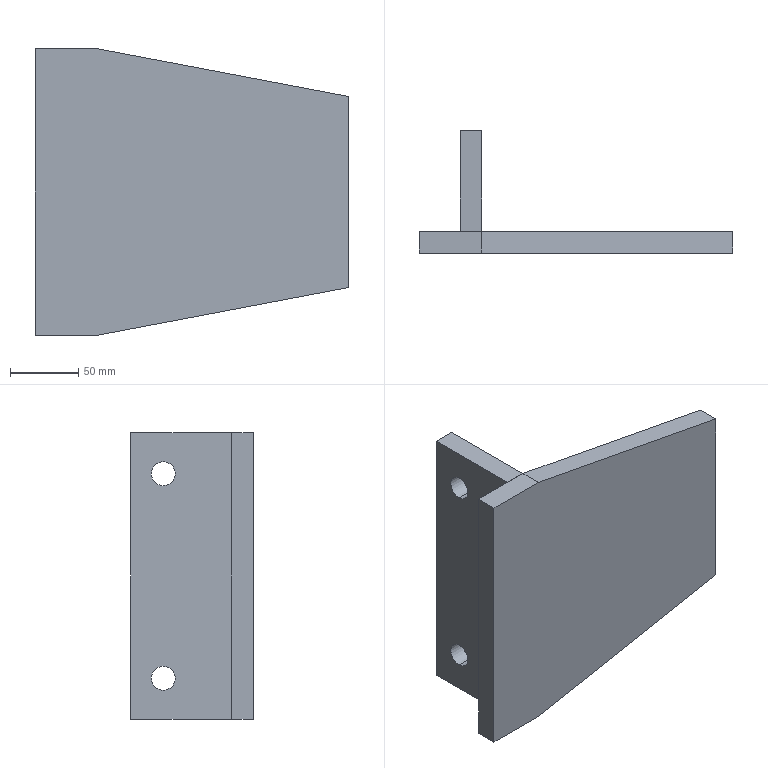Part | SolidWorks | features MirrorStock 1 | 2 solids | 18 faces | box 230 x 90 x 210 mm | volume 910703 mm3 | plane 14 | cylinder 4 | commonest cylinder face diameters 17.5 x4
STEP:
#1=CARTESIAN_POINT('',(46.,0.,105.));
#2=VERTEX_POINT('',#1);
#3=CARTESIAN_POINT('',(0.,0.,105.));
#4=VERTEX_POINT('',#3);
#5=CARTESIAN_POINT('',(46.,0.,105.));
#6=DIRECTION('',(-1.,0.,0.));
#7=VECTOR('',#6,1000.);
#8=LINE('',#5,#7);
#9=EDGE_CURVE('',#2,#4,#8,.T.);
#10=ORIENTED_EDGE('',*,*,#9,.F.);
#11=CARTESIAN_POINT('',(46.,16.,105.));
#12=VERTEX_POINT('',#11);
#13=CARTESIAN_POINT('',(46.,16.,105.));
#14=DIRECTION('',(0.,-1.,0.));
#15=VECTOR('',#14,1000.);
#16=LINE('',#13,#15);
#17=EDGE_CURVE('',#12,#2,#16,.T.);
#18=ORIENTED_EDGE('',*,*,#17,.F.);
#19=CARTESIAN_POINT('',(0.,16.,105.));
#20=VERTEX_POINT('',#19);
#21=CARTESIAN_POINT('',(46.,16.,105.));
#22=DIRECTION('',(-1.,0.,0.));
#23=VECTOR('',#22,1000.);
#24=LINE('',#21,#23);
#25=EDGE_CURVE('',#12,#20,#24,.T.);
#26=ORIENTED_EDGE('',*,*,#25,.T.);
#27=CARTESIAN_POINT('',(0.,16.,105.));
#28=DIRECTION('',(0.,-1.,0.));
#29=VECTOR('',#28,1000.);
#30=LINE('',#27,#29);
#31=EDGE_CURVE('',#20,#4,#30,.T.);
#32=ORIENTED_EDGE('',*,*,#31,.T.);
#33=EDGE_LOOP('',(#10,#18,#26,#32));
#34=FACE_OUTER_BOUND('',#33,.T.);
#35=CARTESIAN_POINT('',(46.,16.,105.));
#36=DIRECTION('',(0.,0.,-1.));
#37=DIRECTION('',(1.,0.,0.));
#38=AXIS2_PLACEMENT_3D('',#35,#36,#37);
#39=PLANE('',#38);
#40=ADVANCED_FACE('',(#34),#39,.F.);
#41=CARTESIAN_POINT('',(0.,0.,-105.));
#42=VERTEX_POINT('',#41);
#43=CARTESIAN_POINT('',(0.,0.,105.));
#44=DIRECTION('',(0.,0.,-1.));
#45=VECTOR('',#44,1000.);
#46=LINE('',#43,#45);
#47=EDGE_CURVE('',#4,#42,#46,.T.);
#48=ORIENTED_EDGE('',*,*,#47,.F.);
#49=ORIENTED_EDGE('',*,*,#31,.F.);
#50=CARTESIAN_POINT('',(0.,16.,-105.));
#51=VERTEX_POINT('',#50);
#52=CARTESIAN_POINT('',(0.,16.,105.));
#53=DIRECTION('',(0.,0.,-1.));
#54=VECTOR('',#53,1000.);
#55=LINE('',#52,#54);
#56=EDGE_CURVE('',#20,#51,#55,.T.);
#57=ORIENTED_EDGE('',*,*,#56,.T.);
#58=CARTESIAN_POINT('',(0.,16.,-105.));
#59=DIRECTION('',(0.,-1.,0.));
#60=VECTOR('',#59,1000.);
#61=LINE('',#58,#60);
#62=EDGE_CURVE('',#51,#42,#61,.T.);
#63=ORIENTED_EDGE('',*,*,#62,.T.);
#64=EDGE_LOOP('',(#48,#49,#57,#63));
#65=FACE_OUTER_BOUND('',#64,.T.);
#66=CARTESIAN_POINT('',(0.,16.,105.));
#67=DIRECTION('',(1.,0.,0.));
#68=DIRECTION('',(0.,0.,1.));
#69=AXIS2_PLACEMENT_3D('',#66,#67,#68);
#70=PLANE('',#69);
#71=ADVANCED_FACE('',(#65),#70,.F.);
#72=CARTESIAN_POINT('',(46.,0.,-105.));
#73=VERTEX_POINT('',#72);
#74=CARTESIAN_POINT('',(46.,0.,-105.));
#75=DIRECTION('',(1.,0.,0.));
#76=VECTOR('',#75,1000.);
#77=LINE('',#74,#76);
#78=EDGE_CURVE('',#42,#73,#77,.T.);
#79=ORIENTED_EDGE('',*,*,#78,.F.);
#80=ORIENTED_EDGE('',*,*,#62,.F.);
#81=CARTESIAN_POINT('',(46.,16.,-105.));
#82=VERTEX_POINT('',#81);
#83=CARTESIAN_POINT('',(46.,16.,-105.));
#84=DIRECTION('',(1.,0.,0.));
#85=VECTOR('',#84,1000.);
#86=LINE('',#83,#85);
#87=EDGE_CURVE('',#51,#82,#86,.T.);
#88=ORIENTED_EDGE('',*,*,#87,.T.);
#89=CARTESIAN_POINT('',(46.,16.,-105.));
#90=DIRECTION('',(0.,-1.,0.));
#91=VECTOR('',#90,1000.);
#92=LINE('',#89,#91);
#93=EDGE_CURVE('',#82,#73,#92,.T.);
#94=ORIENTED_EDGE('',*,*,#93,.T.);
#95=EDGE_LOOP('',(#79,#80,#88,#94));
#96=FACE_OUTER_BOUND('',#95,.T.);
#97=CARTESIAN_POINT('',(46.,16.,-105.));
#98=DIRECTION('',(0.,0.,1.));
#99=DIRECTION('',(-1.,0.,0.));
#100=AXIS2_PLACEMENT_3D('',#97,#98,#99);
#101=PLANE('',#100);
#102=ADVANCED_FACE('',(#96),#101,.F.);
#103=CARTESIAN_POINT('',(230.,0.,-70.));
#104=VERTEX_POINT('',#103);
#105=CARTESIAN_POINT('',(230.,0.,-70.));
#106=DIRECTION('',(0.9824,0.,0.1869));
#107=VECTOR('',#106,1000.);
#108=LINE('',#105,#107);
#109=EDGE_CURVE('',#73,#104,#108,.T.);
#110=ORIENTED_EDGE('',*,*,#109,.F.);
#111=ORIENTED_EDGE('',*,*,#93,.F.);
#112=CARTESIAN_POINT('',(230.,16.,-70.));
#113=VERTEX_POINT('',#112);
#114=CARTESIAN_POINT('',(230.,16.,-70.));
#115=DIRECTION('',(0.9824,0.,0.1869));
#116=VECTOR('',#115,1000.);
#117=LINE('',#114,#116);
#118=EDGE_CURVE('',#82,#113,#117,.T.);
#119=ORIENTED_EDGE('',*,*,#118,.T.);
#120=CARTESIAN_POINT('',(230.,16.,-70.));
#121=DIRECTION('',(0.,-1.,0.));
#122=VECTOR('',#121,1000.);
#123=LINE('',#120,#122);
#124=EDGE_CURVE('',#113,#104,#123,.T.);
#125=ORIENTED_EDGE('',*,*,#124,.T.);
#126=EDGE_LOOP('',(#110,#111,#119,#125));
#127=FACE_OUTER_BOUND('',#126,.T.);
#128=CARTESIAN_POINT('',(230.,16.,-70.));
#129=DIRECTION('',(-0.1869,0.,0.9824));
#130=DIRECTION('',(-0.9824,0.,-0.1869));
#131=AXIS2_PLACEMENT_3D('',#128,#129,#130);
#132=PLANE('',#131);
#133=ADVANCED_FACE('',(#127),#132,.F.);
#134=CARTESIAN_POINT('',(230.,0.,70.));
#135=VERTEX_POINT('',#134);
#136=CARTESIAN_POINT('',(230.,0.,-70.));
#137=DIRECTION('',(0.,0.,1.));
#138=VECTOR('',#137,1000.);
#139=LINE('',#136,#138);
#140=EDGE_CURVE('',#104,#135,#139,.T.);
#141=ORIENTED_EDGE('',*,*,#140,.F.);
#142=ORIENTED_EDGE('',*,*,#124,.F.);
#143=CARTESIAN_POINT('',(230.,16.,70.));
#144=VERTEX_POINT('',#143);
#145=CARTESIAN_POINT('',(230.,16.,-70.));
#146=DIRECTION('',(0.,0.,1.));
#147=VECTOR('',#146,1000.);
#148=LINE('',#145,#147);
#149=EDGE_CURVE('',#113,#144,#148,.T.);
#150=ORIENTED_EDGE('',*,*,#149,.T.);
#151=CARTESIAN_POINT('',(230.,16.,70.));
#152=DIRECTION('',(0.,-1.,0.));
#153=VECTOR('',#152,1000.);
#154=LINE('',#151,#153);
#155=EDGE_CURVE('',#144,#135,#154,.T.);
#156=ORIENTED_EDGE('',*,*,#155,.T.);
#157=EDGE_LOOP('',(#141,#142,#150,#156));
#158=FACE_OUTER_BOUND('',#157,.T.);
#159=CARTESIAN_POINT('',(230.,16.,-70.));
#160=DIRECTION('',(-1.,0.,0.));
#161=DIRECTION('',(0.,0.,-1.));
#162=AXIS2_PLACEMENT_3D('',#159,#160,#161);
#163=PLANE('',#162);
#164=ADVANCED_FACE('',(#158),#163,.F.);
#165=CARTESIAN_POINT('',(230.,0.,70.));
#166=DIRECTION('',(-0.9824,0.,0.1869));
#167=VECTOR('',#166,1000.);
#168=LINE('',#165,#167);
#169=EDGE_CURVE('',#135,#2,#168,.T.);
#170=ORIENTED_EDGE('',*,*,#169,.F.);
#171=ORIENTED_EDGE('',*,*,#155,.F.);
#172=CARTESIAN_POINT('',(230.,16.,70.));
#173=DIRECTION('',(-0.9824,0.,0.1869));
#174=VECTOR('',#173,1000.);
#175=LINE('',#172,#174);
#176=EDGE_CURVE('',#144,#12,#175,.T.);
#177=ORIENTED_EDGE('',*,*,#176,.T.);
#178=ORIENTED_EDGE('',*,*,#17,.T.);
#179=EDGE_LOOP('',(#170,#171,#177,#178));
#180=FACE_OUTER_BOUND('',#179,.T.);
#181=CARTESIAN_POINT('',(230.,16.,70.));
#182=DIRECTION('',(-0.1869,0.,-0.9824));
#183=DIRECTION('',(0.9824,0.,-0.1869));
#184=AXIS2_PLACEMENT_3D('',#181,#182,#183);
#185=PLANE('',#184);
#186=ADVANCED_FACE('',(#180),#185,.F.);
#187=ORIENTED_EDGE('',*,*,#25,.F.);
#188=ORIENTED_EDGE('',*,*,#176,.F.);
#189=ORIENTED_EDGE('',*,*,#149,.F.);
#190=ORIENTED_EDGE('',*,*,#118,.F.);
#191=ORIENTED_EDGE('',*,*,#87,.F.);
#192=ORIENTED_EDGE('',*,*,#56,.F.);
#193=EDGE_LOOP('',(#187,#188,#189,#190,#191,#192));
#194=FACE_OUTER_BOUND('',#193,.T.);
#195=CARTESIAN_POINT('',(0.,16.,0.));
#196=DIRECTION('',(0.,1.,0.));
#197=DIRECTION('',(0.,0.,-1.));
#198=AXIS2_PLACEMENT_3D('',#195,#196,#197);
#199=PLANE('',#198);
#200=ADVANCED_FACE('',(#194),#199,.T.);
#201=ORIENTED_EDGE('',*,*,#9,.T.);
#202=ORIENTED_EDGE('',*,*,#47,.T.);
#203=ORIENTED_EDGE('',*,*,#78,.T.);
#204=ORIENTED_EDGE('',*,*,#109,.T.);
#205=ORIENTED_EDGE('',*,*,#140,.T.);
#206=ORIENTED_EDGE('',*,*,#169,.T.);
#207=EDGE_LOOP('',(#201,#202,#203,#204,#205,#206));
#208=FACE_OUTER_BOUND('',#207,.T.);
#209=CARTESIAN_POINT('',(0.,0.,0.));
#210=DIRECTION('',(0.,1.,0.));
#211=DIRECTION('',(0.,0.,-1.));
#212=AXIS2_PLACEMENT_3D('',#209,#210,#211);
#213=PLANE('',#212);
#214=ADVANCED_FACE('',(#208),#213,.F.);
#215=CLOSED_SHELL('',(#40,#71,#102,#133,#164,#186,#200,#214));
#216=MANIFOLD_SOLID_BREP('',#215);
#217=CARTESIAN_POINT('',(46.,66.,66.25));
#218=VERTEX_POINT('',#217);
#219=CARTESIAN_POINT('',(46.,66.,83.75));
#220=VERTEX_POINT('',#219);
#221=CARTESIAN_POINT('',(46.,66.,75.));
#222=DIRECTION('',(1.,0.,0.));
#223=DIRECTION('',(0.,0.,-1.));
#224=AXIS2_PLACEMENT_3D('',#221,#222,#223);
#225=CIRCLE('',#224,8.75);
#226=EDGE_CURVE('',#218,#220,#225,.T.);
#227=ORIENTED_EDGE('',*,*,#226,.T.);
#228=CARTESIAN_POINT('',(30.,66.,83.75));
#229=VERTEX_POINT('',#228);
#230=CARTESIAN_POINT('',(30.,66.,83.75));
#231=DIRECTION('',(-1.,0.,0.));
#232=VECTOR('',#231,1000.);
#233=LINE('',#230,#232);
#234=EDGE_CURVE('',#220,#229,#233,.T.);
#235=ORIENTED_EDGE('',*,*,#234,.T.);
#236=CARTESIAN_POINT('',(30.,66.,66.25));
#237=VERTEX_POINT('',#236);
#238=CARTESIAN_POINT('',(30.,66.,75.));
#239=DIRECTION('',(1.,0.,0.));
#240=DIRECTION('',(0.,0.,-1.));
#241=AXIS2_PLACEMENT_3D('',#238,#239,#240);
#242=CIRCLE('',#241,8.75);
#243=EDGE_CURVE('',#237,#229,#242,.T.);
#244=ORIENTED_EDGE('',*,*,#243,.F.);
#245=CARTESIAN_POINT('',(30.,66.,66.25));
#246=DIRECTION('',(-1.,0.,0.));
#247=VECTOR('',#246,1000.);
#248=LINE('',#245,#247);
#249=EDGE_CURVE('',#218,#237,#248,.T.);
#250=ORIENTED_EDGE('',*,*,#249,.F.);
#251=EDGE_LOOP('',(#227,#235,#244,#250));
#252=FACE_OUTER_BOUND('',#251,.T.);
#253=CARTESIAN_POINT('',(30.,66.,75.));
#254=DIRECTION('',(-1.,0.,0.));
#255=DIRECTION('',(0.,0.,-1.));
#256=AXIS2_PLACEMENT_3D('',#253,#254,#255);
#257=CYLINDRICAL_SURFACE('',#256,8.75);
#258=ADVANCED_FACE('',(#252),#257,.F.);
#259=CARTESIAN_POINT('',(46.,66.,-83.75));
#260=VERTEX_POINT('',#259);
#261=CARTESIAN_POINT('',(46.,66.,-66.25));
#262=VERTEX_POINT('',#261);
#263=CARTESIAN_POINT('',(46.,66.,-75.));
#264=DIRECTION('',(1.,0.,0.));
#265=DIRECTION('',(0.,0.,-1.));
#266=AXIS2_PLACEMENT_3D('',#263,#264,#265);
#267=CIRCLE('',#266,8.75);
#268=EDGE_CURVE('',#260,#262,#267,.T.);
#269=ORIENTED_EDGE('',*,*,#268,.T.);
#270=CARTESIAN_POINT('',(30.,66.,-66.25));
#271=VERTEX_POINT('',#270);
#272=CARTESIAN_POINT('',(30.,66.,-66.25));
#273=DIRECTION('',(-1.,0.,0.));
#274=VECTOR('',#273,1000.);
#275=LINE('',#272,#274);
#276=EDGE_CURVE('',#262,#271,#275,.T.);
#277=ORIENTED_EDGE('',*,*,#276,.T.);
#278=CARTESIAN_POINT('',(30.,66.,-83.75));
#279=VERTEX_POINT('',#278);
#280=CARTESIAN_POINT('',(30.,66.,-75.));
#281=DIRECTION('',(1.,0.,0.));
#282=DIRECTION('',(0.,0.,-1.));
#283=AXIS2_PLACEMENT_3D('',#280,#281,#282);
#284=CIRCLE('',#283,8.75);
#285=EDGE_CURVE('',#279,#271,#284,.T.);
#286=ORIENTED_EDGE('',*,*,#285,.F.);
#287=CARTESIAN_POINT('',(30.,66.,-83.75));
#288=DIRECTION('',(-1.,0.,0.));
#289=VECTOR('',#288,1000.);
#290=LINE('',#287,#289);
#291=EDGE_CURVE('',#260,#279,#290,.T.);
#292=ORIENTED_EDGE('',*,*,#291,.F.);
#293=EDGE_LOOP('',(#269,#277,#286,#292));
#294=FACE_OUTER_BOUND('',#293,.T.);
#295=CARTESIAN_POINT('',(30.,66.,-75.));
#296=DIRECTION('',(-1.,0.,0.));
#297=DIRECTION('',(0.,0.,-1.));
#298=AXIS2_PLACEMENT_3D('',#295,#296,#297);
#299=CYLINDRICAL_SURFACE('',#298,8.75);
#300=ADVANCED_FACE('',(#294),#299,.F.);
#301=ORIENTED_EDGE('',*,*,#226,.F.);
#302=CARTESIAN_POINT('',(46.,66.,75.));
#303=DIRECTION('',(1.,0.,0.));
#304=DIRECTION('',(0.,0.,-1.));
#305=AXIS2_PLACEMENT_3D('',#302,#303,#304);
#306=CIRCLE('',#305,8.75);
#307=EDGE_CURVE('',#220,#218,#306,.T.);
#308=ORIENTED_EDGE('',*,*,#307,.F.);
#309=EDGE_LOOP('',(#301,#308));
#310=FACE_BOUND('',#309,.T.);
#311=ORIENTED_EDGE('',*,*,#268,.F.);
#312=CARTESIAN_POINT('',(46.,66.,-75.));
#313=DIRECTION('',(1.,0.,0.));
#314=DIRECTION('',(0.,0.,-1.));
#315=AXIS2_PLACEMENT_3D('',#312,#313,#314);
#316=CIRCLE('',#315,8.75);
#317=EDGE_CURVE('',#262,#260,#316,.T.);
#318=ORIENTED_EDGE('',*,*,#317,.F.);
#319=EDGE_LOOP('',(#311,#318));
#320=FACE_BOUND('',#319,.T.);
#321=CARTESIAN_POINT('',(46.,16.,-105.));
#322=VERTEX_POINT('',#321);
#323=CARTESIAN_POINT('',(46.,16.,105.));
#324=VERTEX_POINT('',#323);
#325=CARTESIAN_POINT('',(46.,16.,105.));
#326=DIRECTION('',(0.,0.,1.));
#327=VECTOR('',#326,1000.);
#328=LINE('',#325,#327);
#329=EDGE_CURVE('',#322,#324,#328,.T.);
#330=ORIENTED_EDGE('',*,*,#329,.F.);
#331=CARTESIAN_POINT('',(46.,90.,-105.));
#332=VERTEX_POINT('',#331);
#333=CARTESIAN_POINT('',(46.,90.,-105.));
#334=DIRECTION('',(0.,-1.,0.));
#335=VECTOR('',#334,1000.);
#336=LINE('',#333,#335);
#337=EDGE_CURVE('',#332,#322,#336,.T.);
#338=ORIENTED_EDGE('',*,*,#337,.F.);
#339=CARTESIAN_POINT('',(46.,90.,105.));
#340=VERTEX_POINT('',#339);
#341=CARTESIAN_POINT('',(46.,90.,105.));
#342=DIRECTION('',(0.,0.,1.));
#343=VECTOR('',#342,1000.);
#344=LINE('',#341,#343);
#345=EDGE_CURVE('',#332,#340,#344,.T.);
#346=ORIENTED_EDGE('',*,*,#345,.T.);
#347=CARTESIAN_POINT('',(46.,90.,105.));
#348=DIRECTION('',(0.,-1.,0.));
#349=VECTOR('',#348,1000.);
#350=LINE('',#347,#349);
#351=EDGE_CURVE('',#340,#324,#350,.T.);
#352=ORIENTED_EDGE('',*,*,#351,.T.);
#353=EDGE_LOOP('',(#330,#338,#346,#352));
#354=FACE_OUTER_BOUND('',#353,.T.);
#355=CARTESIAN_POINT('',(46.,90.,105.));
#356=DIRECTION('',(-1.,0.,0.));
#357=DIRECTION('',(0.,0.,-1.));
#358=AXIS2_PLACEMENT_3D('',#355,#356,#357);
#359=PLANE('',#358);
#360=ADVANCED_FACE('',(#310,#320,#354),#359,.F.);
#361=CARTESIAN_POINT('',(30.,16.,105.));
#362=VERTEX_POINT('',#361);
#363=CARTESIAN_POINT('',(46.,16.,105.));
#364=DIRECTION('',(-1.,0.,0.));
#365=VECTOR('',#364,1000.);
#366=LINE('',#363,#365);
#367=EDGE_CURVE('',#324,#362,#366,.T.);
#368=ORIENTED_EDGE('',*,*,#367,.F.);
#369=ORIENTED_EDGE('',*,*,#351,.F.);
#370=CARTESIAN_POINT('',(30.,90.,105.));
#371=VERTEX_POINT('',#370);
#372=CARTESIAN_POINT('',(46.,90.,105.));
#373=DIRECTION('',(-1.,0.,0.));
#374=VECTOR('',#373,1000.);
#375=LINE('',#372,#374);
#376=EDGE_CURVE('',#340,#371,#375,.T.);
#377=ORIENTED_EDGE('',*,*,#376,.T.);
#378=CARTESIAN_POINT('',(30.,90.,105.));
#379=DIRECTION('',(0.,-1.,0.));
#380=VECTOR('',#379,1000.);
#381=LINE('',#378,#380);
#382=EDGE_CURVE('',#371,#362,#381,.T.);
#383=ORIENTED_EDGE('',*,*,#382,.T.);
#384=EDGE_LOOP('',(#368,#369,#377,#383));
#385=FACE_OUTER_BOUND('',#384,.T.);
#386=CARTESIAN_POINT('',(46.,90.,105.));
#387=DIRECTION('',(0.,0.,-1.));
#388=DIRECTION('',(1.,0.,0.));
#389=AXIS2_PLACEMENT_3D('',#386,#387,#388);
#390=PLANE('',#389);
#391=ADVANCED_FACE('',(#385),#390,.F.);
#392=ORIENTED_EDGE('',*,*,#243,.T.);
#393=CARTESIAN_POINT('',(30.,66.,75.));
#394=DIRECTION('',(1.,0.,0.));
#395=DIRECTION('',(0.,0.,-1.));
#396=AXIS2_PLACEMENT_3D('',#393,#394,#395);
#397=CIRCLE('',#396,8.75);
#398=EDGE_CURVE('',#229,#237,#397,.T.);
#399=ORIENTED_EDGE('',*,*,#398,.T.);
#400=EDGE_LOOP('',(#392,#399));
#401=FACE_BOUND('',#400,.T.);
#402=ORIENTED_EDGE('',*,*,#285,.T.);
#403=CARTESIAN_POINT('',(30.,66.,-75.));
#404=DIRECTION('',(1.,0.,0.));
#405=DIRECTION('',(0.,0.,-1.));
#406=AXIS2_PLACEMENT_3D('',#403,#404,#405);
#407=CIRCLE('',#406,8.75);
#408=EDGE_CURVE('',#271,#279,#407,.T.);
#409=ORIENTED_EDGE('',*,*,#408,.T.);
#410=EDGE_LOOP('',(#402,#409));
#411=FACE_BOUND('',#410,.T.);
#412=CARTESIAN_POINT('',(30.,16.,-105.));
#413=VERTEX_POINT('',#412);
#414=CARTESIAN_POINT('',(30.,16.,105.));
#415=DIRECTION('',(0.,0.,-1.));
#416=VECTOR('',#415,1000.);
#417=LINE('',#414,#416);
#418=EDGE_CURVE('',#362,#413,#417,.T.);
#419=ORIENTED_EDGE('',*,*,#418,.F.);
#420=ORIENTED_EDGE('',*,*,#382,.F.);
#421=CARTESIAN_POINT('',(30.,90.,-105.));
#422=VERTEX_POINT('',#421);
#423=CARTESIAN_POINT('',(30.,90.,105.));
#424=DIRECTION('',(0.,0.,-1.));
#425=VECTOR('',#424,1000.);
#426=LINE('',#423,#425);
#427=EDGE_CURVE('',#371,#422,#426,.T.);
#428=ORIENTED_EDGE('',*,*,#427,.T.);
#429=CARTESIAN_POINT('',(30.,90.,-105.));
#430=DIRECTION('',(0.,-1.,0.));
#431=VECTOR('',#430,1000.);
#432=LINE('',#429,#431);
#433=EDGE_CURVE('',#422,#413,#432,.T.);
#434=ORIENTED_EDGE('',*,*,#433,.T.);
#435=EDGE_LOOP('',(#419,#420,#428,#434));
#436=FACE_OUTER_BOUND('',#435,.T.);
#437=CARTESIAN_POINT('',(30.,90.,105.));
#438=DIRECTION('',(1.,0.,0.));
#439=DIRECTION('',(0.,0.,1.));
#440=AXIS2_PLACEMENT_3D('',#437,#438,#439);
#441=PLANE('',#440);
#442=ADVANCED_FACE('',(#401,#411,#436),#441,.F.);
#443=CARTESIAN_POINT('',(46.,16.,-105.));
#444=DIRECTION('',(1.,0.,0.));
#445=VECTOR('',#444,1000.);
#446=LINE('',#443,#445);
#447=EDGE_CURVE('',#413,#322,#446,.T.);
#448=ORIENTED_EDGE('',*,*,#447,.F.);
#449=ORIENTED_EDGE('',*,*,#433,.F.);
#450=CARTESIAN_POINT('',(46.,90.,-105.));
#451=DIRECTION('',(1.,0.,0.));
#452=VECTOR('',#451,1000.);
#453=LINE('',#450,#452);
#454=EDGE_CURVE('',#422,#332,#453,.T.);
#455=ORIENTED_EDGE('',*,*,#454,.T.);
#456=ORIENTED_EDGE('',*,*,#337,.T.);
#457=EDGE_LOOP('',(#448,#449,#455,#456));
#458=FACE_OUTER_BOUND('',#457,.T.);
#459=CARTESIAN_POINT('',(46.,90.,-105.));
#460=DIRECTION('',(0.,0.,1.));
#461=DIRECTION('',(-1.,0.,0.));
#462=AXIS2_PLACEMENT_3D('',#459,#460,#461);
#463=PLANE('',#462);
#464=ADVANCED_FACE('',(#458),#463,.F.);
#465=ORIENTED_EDGE('',*,*,#345,.F.);
#466=ORIENTED_EDGE('',*,*,#454,.F.);
#467=ORIENTED_EDGE('',*,*,#427,.F.);
#468=ORIENTED_EDGE('',*,*,#376,.F.);
#469=EDGE_LOOP('',(#465,#466,#467,#468));
#470=FACE_OUTER_BOUND('',#469,.T.);
#471=CARTESIAN_POINT('',(0.,90.,0.));
#472=DIRECTION('',(0.,-1.,0.));
#473=DIRECTION('',(0.,0.,1.));
#474=AXIS2_PLACEMENT_3D('',#471,#472,#473);
#475=PLANE('',#474);
#476=ADVANCED_FACE('',(#470),#475,.F.);
#477=ORIENTED_EDGE('',*,*,#329,.T.);
#478=ORIENTED_EDGE('',*,*,#367,.T.);
#479=ORIENTED_EDGE('',*,*,#418,.T.);
#480=ORIENTED_EDGE('',*,*,#447,.T.);
#481=EDGE_LOOP('',(#477,#478,#479,#480));
#482=FACE_OUTER_BOUND('',#481,.T.);
#483=CARTESIAN_POINT('',(0.,16.,0.));
#484=DIRECTION('',(0.,-1.,0.));
#485=DIRECTION('',(0.,0.,1.));
#486=AXIS2_PLACEMENT_3D('',#483,#484,#485);
#487=PLANE('',#486);
#488=ADVANCED_FACE('',(#482),#487,.T.);
#489=ORIENTED_EDGE('',*,*,#276,.F.);
#490=ORIENTED_EDGE('',*,*,#317,.T.);
#491=ORIENTED_EDGE('',*,*,#291,.T.);
#492=ORIENTED_EDGE('',*,*,#408,.F.);
#493=EDGE_LOOP('',(#489,#490,#491,#492));
#494=FACE_OUTER_BOUND('',#493,.T.);
#495=CARTESIAN_POINT('',(30.,66.,-75.));
#496=DIRECTION('',(-1.,0.,0.));
#497=DIRECTION('',(0.,0.,-1.));
#498=AXIS2_PLACEMENT_3D('',#495,#496,#497);
#499=CYLINDRICAL_SURFACE('',#498,8.75);
#500=ADVANCED_FACE('',(#494),#499,.F.);
#501=ORIENTED_EDGE('',*,*,#234,.F.);
#502=ORIENTED_EDGE('',*,*,#307,.T.);
#503=ORIENTED_EDGE('',*,*,#249,.T.);
#504=ORIENTED_EDGE('',*,*,#398,.F.);
#505=EDGE_LOOP('',(#501,#502,#503,#504));
#506=FACE_OUTER_BOUND('',#505,.T.);
#507=CARTESIAN_POINT('',(30.,66.,75.));
#508=DIRECTION('',(-1.,0.,0.));
#509=DIRECTION('',(0.,0.,-1.));
#510=AXIS2_PLACEMENT_3D('',#507,#508,#509);
#511=CYLINDRICAL_SURFACE('',#510,8.75);
#512=ADVANCED_FACE('',(#506),#511,.F.);
#513=CLOSED_SHELL('',(#258,#300,#360,#391,#442,#464,#476,#488,#500,#512));
#514=MANIFOLD_SOLID_BREP('',#513);
#515=CARTESIAN_POINT('',(0.,0.,0.));
#516=DIRECTION('',(0.,0.,1.));
#517=DIRECTION('',(1.,0.,0.));
#518=AXIS2_PLACEMENT_3D('',#515,#516,#517);
#519=(LENGTH_UNIT()NAMED_UNIT(*)SI_UNIT(.MILLI.,.METRE.));
#520=UNCERTAINTY_MEASURE_WITH_UNIT(LENGTH_MEASURE(0.00001),#519,'','');
#521=(NAMED_UNIT(*)PLANE_ANGLE_UNIT()SI_UNIT($,.RADIAN.));
#522=(NAMED_UNIT(*)SI_UNIT($,.STERADIAN.)SOLID_ANGLE_UNIT());
#523=(GEOMETRIC_REPRESENTATION_CONTEXT(3)GLOBAL_UNCERTAINTY_ASSIGNED_CONTEXT((#520))GLOBAL_UNIT_ASSIGNED_CONTEXT((#519,#521,#522))REPRESENTATION_CONTEXT('',''));
#524=ADVANCED_BREP_SHAPE_REPRESENTATION('',(#216,#514,#518),#523);